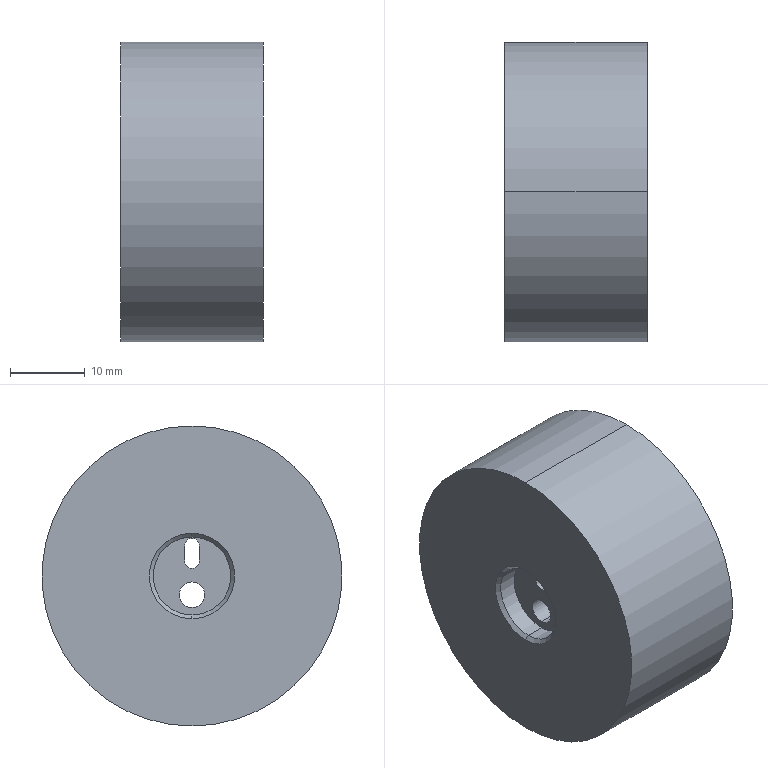Part | SolidWorks | features ICE 3, Chamfer 2, HoleWzd 1, Revolution 1 | 1 solid | 28 faces | box 19 x 40 x 40 mm | volume 21751 mm3 | plane 15 | cylinder 11 | cone 2 | commonest cylinder face diameters 2 x3 3.4 x2 6.5 x2 10.4 x2 40 x2
STEP:
#1=CARTESIAN_POINT('',(0.5,0.,-5.2));
#2=VERTEX_POINT('',#1);
#3=CARTESIAN_POINT('',(0.5,0.,5.2));
#4=VERTEX_POINT('',#3);
#5=CARTESIAN_POINT('',(0.5,0.,0.));
#6=DIRECTION('',(-1.,0.,0.));
#7=DIRECTION('',(0.,0.,1.));
#8=AXIS2_PLACEMENT_3D('',#5,#6,#7);
#9=CIRCLE('',#8,5.2);
#10=EDGE_CURVE('',#2,#4,#9,.T.);
#11=ORIENTED_EDGE('',*,*,#10,.F.);
#12=CARTESIAN_POINT('',(0.,0.,-5.7));
#13=VERTEX_POINT('',#12);
#14=CARTESIAN_POINT('',(0.5,0.,-5.2));
#15=DIRECTION('',(-0.7071,0.,-0.7071));
#16=VECTOR('',#15,1000.);
#17=LINE('',#14,#16);
#18=EDGE_CURVE('',#2,#13,#17,.T.);
#19=ORIENTED_EDGE('',*,*,#18,.T.);
#20=CARTESIAN_POINT('',(0.,0.,5.7));
#21=VERTEX_POINT('',#20);
#22=CARTESIAN_POINT('',(0.,0.,0.));
#23=DIRECTION('',(1.,0.,0.));
#24=DIRECTION('',(0.,0.,1.));
#25=AXIS2_PLACEMENT_3D('',#22,#23,#24);
#26=CIRCLE('',#25,5.7);
#27=EDGE_CURVE('',#21,#13,#26,.T.);
#28=ORIENTED_EDGE('',*,*,#27,.F.);
#29=CARTESIAN_POINT('',(0.5,0.,5.2));
#30=DIRECTION('',(-0.7071,0.,0.7071));
#31=VECTOR('',#30,1000.);
#32=LINE('',#29,#31);
#33=EDGE_CURVE('',#4,#21,#32,.T.);
#34=ORIENTED_EDGE('',*,*,#33,.F.);
#35=EDGE_LOOP('',(#11,#19,#28,#34));
#36=FACE_OUTER_BOUND('',#35,.T.);
#37=CARTESIAN_POINT('',(0.5,0.,0.));
#38=DIRECTION('',(-1.,0.,0.));
#39=DIRECTION('',(0.,0.,1.));
#40=AXIS2_PLACEMENT_3D('',#37,#38,#39);
#41=CONICAL_SURFACE('',#40,5.2,0.7854);
#42=ADVANCED_FACE('',(#36),#41,.F.);
#43=CARTESIAN_POINT('',(3.,0.,-5.2));
#44=VERTEX_POINT('',#43);
#45=CARTESIAN_POINT('',(3.,0.,5.2));
#46=VERTEX_POINT('',#45);
#47=CARTESIAN_POINT('',(3.,0.,0.));
#48=DIRECTION('',(-1.,0.,0.));
#49=DIRECTION('',(0.,0.,1.));
#50=AXIS2_PLACEMENT_3D('',#47,#48,#49);
#51=CIRCLE('',#50,5.2);
#52=EDGE_CURVE('',#44,#46,#51,.T.);
#53=ORIENTED_EDGE('',*,*,#52,.F.);
#54=CARTESIAN_POINT('',(3.,0.,-5.2));
#55=DIRECTION('',(-1.,0.,0.));
#56=VECTOR('',#55,1000.);
#57=LINE('',#54,#56);
#58=EDGE_CURVE('',#44,#2,#57,.T.);
#59=ORIENTED_EDGE('',*,*,#58,.T.);
#60=ORIENTED_EDGE('',*,*,#10,.T.);
#61=CARTESIAN_POINT('',(3.,0.,5.2));
#62=DIRECTION('',(-1.,0.,0.));
#63=VECTOR('',#62,1000.);
#64=LINE('',#61,#63);
#65=EDGE_CURVE('',#46,#4,#64,.T.);
#66=ORIENTED_EDGE('',*,*,#65,.F.);
#67=EDGE_LOOP('',(#53,#59,#60,#66));
#68=FACE_OUTER_BOUND('',#67,.T.);
#69=CARTESIAN_POINT('',(3.,0.,0.));
#70=DIRECTION('',(-1.,0.,0.));
#71=DIRECTION('',(0.,0.,1.));
#72=AXIS2_PLACEMENT_3D('',#69,#70,#71);
#73=CYLINDRICAL_SURFACE('',#72,5.2);
#74=ADVANCED_FACE('',(#68),#73,.F.);
#75=CARTESIAN_POINT('',(6.5,0.,0.75));
#76=VERTEX_POINT('',#75);
#77=CARTESIAN_POINT('',(6.5,0.,-5.75));
#78=VERTEX_POINT('',#77);
#79=CARTESIAN_POINT('',(6.5,0.,-2.5));
#80=DIRECTION('',(1.,0.,0.));
#81=DIRECTION('',(0.,0.,-1.));
#82=AXIS2_PLACEMENT_3D('',#79,#80,#81);
#83=CIRCLE('',#82,3.25);
#84=EDGE_CURVE('',#76,#78,#83,.T.);
#85=ORIENTED_EDGE('',*,*,#84,.F.);
#86=CARTESIAN_POINT('',(10.,0.,0.75));
#87=VERTEX_POINT('',#86);
#88=CARTESIAN_POINT('',(10.,0.,0.75));
#89=DIRECTION('',(1.,0.,0.));
#90=VECTOR('',#89,1000.);
#91=LINE('',#88,#90);
#92=EDGE_CURVE('',#76,#87,#91,.T.);
#93=ORIENTED_EDGE('',*,*,#92,.T.);
#94=CARTESIAN_POINT('',(10.,0.,-5.75));
#95=VERTEX_POINT('',#94);
#96=CARTESIAN_POINT('',(10.,0.,-2.5));
#97=DIRECTION('',(1.,0.,0.));
#98=DIRECTION('',(0.,0.,-1.));
#99=AXIS2_PLACEMENT_3D('',#96,#97,#98);
#100=CIRCLE('',#99,3.25);
#101=EDGE_CURVE('',#87,#95,#100,.T.);
#102=ORIENTED_EDGE('',*,*,#101,.T.);
#103=CARTESIAN_POINT('',(10.,0.,-5.75));
#104=DIRECTION('',(1.,0.,0.));
#105=VECTOR('',#104,1000.);
#106=LINE('',#103,#105);
#107=EDGE_CURVE('',#78,#95,#106,.T.);
#108=ORIENTED_EDGE('',*,*,#107,.F.);
#109=EDGE_LOOP('',(#85,#93,#102,#108));
#110=FACE_OUTER_BOUND('',#109,.T.);
#111=CARTESIAN_POINT('',(10.,0.,-2.5));
#112=DIRECTION('',(1.,0.,0.));
#113=DIRECTION('',(0.,0.,-1.));
#114=AXIS2_PLACEMENT_3D('',#111,#112,#113);
#115=CYLINDRICAL_SURFACE('',#114,3.25);
#116=ADVANCED_FACE('',(#110),#115,.F.);
#117=CARTESIAN_POINT('',(19.,0.,20.));
#118=VERTEX_POINT('',#117);
#119=CARTESIAN_POINT('',(19.,0.,-20.));
#120=VERTEX_POINT('',#119);
#121=CARTESIAN_POINT('',(19.,0.,0.));
#122=DIRECTION('',(-1.,0.,0.));
#123=DIRECTION('',(0.,0.,1.));
#124=AXIS2_PLACEMENT_3D('',#121,#122,#123);
#125=CIRCLE('',#124,20.);
#126=EDGE_CURVE('',#118,#120,#125,.T.);
#127=ORIENTED_EDGE('',*,*,#126,.T.);
#128=CARTESIAN_POINT('',(0.,0.,-20.));
#129=VERTEX_POINT('',#128);
#130=CARTESIAN_POINT('',(0.,0.,-20.));
#131=DIRECTION('',(-1.,0.,0.));
#132=VECTOR('',#131,1000.);
#133=LINE('',#130,#132);
#134=EDGE_CURVE('',#120,#129,#133,.T.);
#135=ORIENTED_EDGE('',*,*,#134,.T.);
#136=CARTESIAN_POINT('',(0.,0.,20.));
#137=VERTEX_POINT('',#136);
#138=CARTESIAN_POINT('',(0.,0.,0.));
#139=DIRECTION('',(-1.,0.,0.));
#140=DIRECTION('',(0.,0.,1.));
#141=AXIS2_PLACEMENT_3D('',#138,#139,#140);
#142=CIRCLE('',#141,20.);
#143=EDGE_CURVE('',#137,#129,#142,.T.);
#144=ORIENTED_EDGE('',*,*,#143,.F.);
#145=CARTESIAN_POINT('',(0.,0.,20.));
#146=DIRECTION('',(-1.,0.,0.));
#147=VECTOR('',#146,1000.);
#148=LINE('',#145,#147);
#149=EDGE_CURVE('',#118,#137,#148,.T.);
#150=ORIENTED_EDGE('',*,*,#149,.F.);
#151=EDGE_LOOP('',(#127,#135,#144,#150));
#152=FACE_OUTER_BOUND('',#151,.T.);
#153=CARTESIAN_POINT('',(0.,0.,0.));
#154=DIRECTION('',(-1.,0.,0.));
#155=DIRECTION('',(0.,0.,1.));
#156=AXIS2_PLACEMENT_3D('',#153,#154,#155);
#157=CYLINDRICAL_SURFACE('',#156,20.);
#158=ADVANCED_FACE('',(#152),#157,.T.);
#159=CARTESIAN_POINT('',(3.,0.,1.));
#160=VERTEX_POINT('',#159);
#161=CARTESIAN_POINT('',(3.,1.,2.));
#162=VERTEX_POINT('',#161);
#163=CARTESIAN_POINT('',(3.,0.,2.));
#164=DIRECTION('',(1.,0.,0.));
#165=DIRECTION('',(0.,0.,1.));
#166=AXIS2_PLACEMENT_3D('',#163,#164,#165);
#167=CIRCLE('',#166,1.);
#168=EDGE_CURVE('',#160,#162,#167,.T.);
#169=ORIENTED_EDGE('',*,*,#168,.F.);
#170=CARTESIAN_POINT('',(10.,0.,1.));
#171=VERTEX_POINT('',#170);
#172=CARTESIAN_POINT('',(0.,0.,1.));
#173=DIRECTION('',(1.,0.,0.));
#174=VECTOR('',#173,1000.);
#175=LINE('',#172,#174);
#176=EDGE_CURVE('',#160,#171,#175,.T.);
#177=ORIENTED_EDGE('',*,*,#176,.T.);
#178=CARTESIAN_POINT('',(10.,1.,2.));
#179=VERTEX_POINT('',#178);
#180=CARTESIAN_POINT('',(10.,0.,2.));
#181=DIRECTION('',(1.,0.,0.));
#182=DIRECTION('',(0.,0.,-1.));
#183=AXIS2_PLACEMENT_3D('',#180,#181,#182);
#184=CIRCLE('',#183,1.);
#185=EDGE_CURVE('',#171,#179,#184,.T.);
#186=ORIENTED_EDGE('',*,*,#185,.T.);
#187=CARTESIAN_POINT('',(0.,1.,2.));
#188=DIRECTION('',(1.,0.,0.));
#189=VECTOR('',#188,1000.);
#190=LINE('',#187,#189);
#191=EDGE_CURVE('',#162,#179,#190,.T.);
#192=ORIENTED_EDGE('',*,*,#191,.F.);
#193=EDGE_LOOP('',(#169,#177,#186,#192));
#194=FACE_OUTER_BOUND('',#193,.T.);
#195=CARTESIAN_POINT('',(0.,0.,2.));
#196=DIRECTION('',(1.,0.,0.));
#197=DIRECTION('',(0.,0.,-1.));
#198=AXIS2_PLACEMENT_3D('',#195,#196,#197);
#199=CYLINDRICAL_SURFACE('',#198,1.);
#200=ADVANCED_FACE('',(#194),#199,.F.);
#201=CARTESIAN_POINT('',(3.,0.,-0.8));
#202=VERTEX_POINT('',#201);
#203=CARTESIAN_POINT('',(3.,0.,-4.2));
#204=VERTEX_POINT('',#203);
#205=CARTESIAN_POINT('',(3.,0.,-2.5));
#206=DIRECTION('',(1.,0.,0.));
#207=DIRECTION('',(0.,0.,1.));
#208=AXIS2_PLACEMENT_3D('',#205,#206,#207);
#209=CIRCLE('',#208,1.7);
#210=EDGE_CURVE('',#202,#204,#209,.T.);
#211=ORIENTED_EDGE('',*,*,#210,.F.);
#212=CARTESIAN_POINT('',(6.5,0.,-0.8));
#213=VERTEX_POINT('',#212);
#214=CARTESIAN_POINT('',(10.,0.,-0.8));
#215=DIRECTION('',(1.,0.,0.));
#216=VECTOR('',#215,1000.);
#217=LINE('',#214,#216);
#218=EDGE_CURVE('',#202,#213,#217,.T.);
#219=ORIENTED_EDGE('',*,*,#218,.T.);
#220=CARTESIAN_POINT('',(6.5,0.,-4.2));
#221=VERTEX_POINT('',#220);
#222=CARTESIAN_POINT('',(6.5,0.,-2.5));
#223=DIRECTION('',(1.,0.,0.));
#224=DIRECTION('',(0.,0.,-1.));
#225=AXIS2_PLACEMENT_3D('',#222,#223,#224);
#226=CIRCLE('',#225,1.7);
#227=EDGE_CURVE('',#213,#221,#226,.T.);
#228=ORIENTED_EDGE('',*,*,#227,.T.);
#229=CARTESIAN_POINT('',(10.,0.,-4.2));
#230=DIRECTION('',(1.,0.,0.));
#231=VECTOR('',#230,1000.);
#232=LINE('',#229,#231);
#233=EDGE_CURVE('',#204,#221,#232,.T.);
#234=ORIENTED_EDGE('',*,*,#233,.F.);
#235=EDGE_LOOP('',(#211,#219,#228,#234));
#236=FACE_OUTER_BOUND('',#235,.T.);
#237=CARTESIAN_POINT('',(10.,0.,-2.5));
#238=DIRECTION('',(1.,0.,0.));
#239=DIRECTION('',(0.,0.,-1.));
#240=AXIS2_PLACEMENT_3D('',#237,#238,#239);
#241=CYLINDRICAL_SURFACE('',#240,1.7);
#242=ADVANCED_FACE('',(#236),#241,.F.);
#243=ORIENTED_EDGE('',*,*,#218,.F.);
#244=CARTESIAN_POINT('',(3.,0.,-2.5));
#245=DIRECTION('',(1.,0.,0.));
#246=DIRECTION('',(0.,0.,1.));
#247=AXIS2_PLACEMENT_3D('',#244,#245,#246);
#248=CIRCLE('',#247,1.7);
#249=EDGE_CURVE('',#204,#202,#248,.T.);
#250=ORIENTED_EDGE('',*,*,#249,.F.);
#251=ORIENTED_EDGE('',*,*,#233,.T.);
#252=CARTESIAN_POINT('',(6.5,0.,-2.5));
#253=DIRECTION('',(1.,0.,0.));
#254=DIRECTION('',(0.,0.,-1.));
#255=AXIS2_PLACEMENT_3D('',#252,#253,#254);
#256=CIRCLE('',#255,1.7);
#257=EDGE_CURVE('',#221,#213,#256,.T.);
#258=ORIENTED_EDGE('',*,*,#257,.T.);
#259=EDGE_LOOP('',(#243,#250,#251,#258));
#260=FACE_OUTER_BOUND('',#259,.T.);
#261=CARTESIAN_POINT('',(10.,0.,-2.5));
#262=DIRECTION('',(1.,0.,0.));
#263=DIRECTION('',(0.,0.,-1.));
#264=AXIS2_PLACEMENT_3D('',#261,#262,#263);
#265=CYLINDRICAL_SURFACE('',#264,1.7);
#266=ADVANCED_FACE('',(#260),#265,.F.);
#267=ORIENTED_EDGE('',*,*,#176,.F.);
#268=CARTESIAN_POINT('',(3.,-1.,2.));
#269=VERTEX_POINT('',#268);
#270=CARTESIAN_POINT('',(3.,0.,2.));
#271=DIRECTION('',(1.,0.,0.));
#272=DIRECTION('',(0.,0.,1.));
#273=AXIS2_PLACEMENT_3D('',#270,#271,#272);
#274=CIRCLE('',#273,1.);
#275=EDGE_CURVE('',#269,#160,#274,.T.);
#276=ORIENTED_EDGE('',*,*,#275,.F.);
#277=CARTESIAN_POINT('',(10.,-1.,2.));
#278=VERTEX_POINT('',#277);
#279=CARTESIAN_POINT('',(0.,-1.,2.));
#280=DIRECTION('',(1.,0.,0.));
#281=VECTOR('',#280,1000.);
#282=LINE('',#279,#281);
#283=EDGE_CURVE('',#269,#278,#282,.T.);
#284=ORIENTED_EDGE('',*,*,#283,.T.);
#285=CARTESIAN_POINT('',(10.,0.,2.));
#286=DIRECTION('',(1.,0.,0.));
#287=DIRECTION('',(0.,0.,-1.));
#288=AXIS2_PLACEMENT_3D('',#285,#286,#287);
#289=CIRCLE('',#288,1.);
#290=EDGE_CURVE('',#278,#171,#289,.T.);
#291=ORIENTED_EDGE('',*,*,#290,.T.);
#292=EDGE_LOOP('',(#267,#276,#284,#291));
#293=FACE_OUTER_BOUND('',#292,.T.);
#294=CARTESIAN_POINT('',(0.,0.,2.));
#295=DIRECTION('',(1.,0.,0.));
#296=DIRECTION('',(0.,0.,-1.));
#297=AXIS2_PLACEMENT_3D('',#294,#295,#296);
#298=CYLINDRICAL_SURFACE('',#297,1.);
#299=ADVANCED_FACE('',(#293),#298,.F.);
#300=CARTESIAN_POINT('',(3.,-1.,4.));
#301=VERTEX_POINT('',#300);
#302=CARTESIAN_POINT('',(3.,-1.,2.));
#303=DIRECTION('',(0.,0.,-1.));
#304=VECTOR('',#303,1000.);
#305=LINE('',#302,#304);
#306=EDGE_CURVE('',#301,#269,#305,.T.);
#307=ORIENTED_EDGE('',*,*,#306,.F.);
#308=CARTESIAN_POINT('',(10.,-1.,4.));
#309=VERTEX_POINT('',#308);
#310=CARTESIAN_POINT('',(0.,-1.,4.));
#311=DIRECTION('',(1.,0.,0.));
#312=VECTOR('',#311,1000.);
#313=LINE('',#310,#312);
#314=EDGE_CURVE('',#301,#309,#313,.T.);
#315=ORIENTED_EDGE('',*,*,#314,.T.);
#316=CARTESIAN_POINT('',(10.,-1.,2.));
#317=DIRECTION('',(0.,0.,-1.));
#318=VECTOR('',#317,1000.);
#319=LINE('',#316,#318);
#320=EDGE_CURVE('',#309,#278,#319,.T.);
#321=ORIENTED_EDGE('',*,*,#320,.T.);
#322=ORIENTED_EDGE('',*,*,#283,.F.);
#323=EDGE_LOOP('',(#307,#315,#321,#322));
#324=FACE_OUTER_BOUND('',#323,.T.);
#325=CARTESIAN_POINT('',(0.,-1.,2.));
#326=DIRECTION('',(0.,-1.,0.));
#327=DIRECTION('',(0.,0.,-1.));
#328=AXIS2_PLACEMENT_3D('',#325,#326,#327);
#329=PLANE('',#328);
#330=ADVANCED_FACE('',(#324),#329,.F.);
#331=CARTESIAN_POINT('',(3.,1.,4.));
#332=VERTEX_POINT('',#331);
#333=CARTESIAN_POINT('',(3.,0.,4.));
#334=DIRECTION('',(1.,0.,0.));
#335=DIRECTION('',(0.,0.,1.));
#336=AXIS2_PLACEMENT_3D('',#333,#334,#335);
#337=CIRCLE('',#336,1.);
#338=EDGE_CURVE('',#332,#301,#337,.T.);
#339=ORIENTED_EDGE('',*,*,#338,.F.);
#340=CARTESIAN_POINT('',(10.,1.,4.));
#341=VERTEX_POINT('',#340);
#342=CARTESIAN_POINT('',(0.,1.,4.));
#343=DIRECTION('',(1.,0.,0.));
#344=VECTOR('',#343,1000.);
#345=LINE('',#342,#344);
#346=EDGE_CURVE('',#332,#341,#345,.T.);
#347=ORIENTED_EDGE('',*,*,#346,.T.);
#348=CARTESIAN_POINT('',(10.,0.,4.));
#349=DIRECTION('',(1.,0.,0.));
#350=DIRECTION('',(0.,0.,-1.));
#351=AXIS2_PLACEMENT_3D('',#348,#349,#350);
#352=CIRCLE('',#351,1.);
#353=EDGE_CURVE('',#341,#309,#352,.T.);
#354=ORIENTED_EDGE('',*,*,#353,.T.);
#355=ORIENTED_EDGE('',*,*,#314,.F.);
#356=EDGE_LOOP('',(#339,#347,#354,#355));
#357=FACE_OUTER_BOUND('',#356,.T.);
#358=CARTESIAN_POINT('',(0.,0.,4.));
#359=DIRECTION('',(1.,0.,0.));
#360=DIRECTION('',(0.,0.,-1.));
#361=AXIS2_PLACEMENT_3D('',#358,#359,#360);
#362=CYLINDRICAL_SURFACE('',#361,1.);
#363=ADVANCED_FACE('',(#357),#362,.F.);
#364=CARTESIAN_POINT('',(3.,1.,2.));
#365=DIRECTION('',(0.,0.,1.));
#366=VECTOR('',#365,1000.);
#367=LINE('',#364,#366);
#368=EDGE_CURVE('',#162,#332,#367,.T.);
#369=ORIENTED_EDGE('',*,*,#368,.F.);
#370=ORIENTED_EDGE('',*,*,#191,.T.);
#371=CARTESIAN_POINT('',(10.,1.,2.));
#372=DIRECTION('',(0.,0.,1.));
#373=VECTOR('',#372,1000.);
#374=LINE('',#371,#373);
#375=EDGE_CURVE('',#179,#341,#374,.T.);
#376=ORIENTED_EDGE('',*,*,#375,.T.);
#377=ORIENTED_EDGE('',*,*,#346,.F.);
#378=EDGE_LOOP('',(#369,#370,#376,#377));
#379=FACE_OUTER_BOUND('',#378,.T.);
#380=CARTESIAN_POINT('',(0.,1.,2.));
#381=DIRECTION('',(0.,1.,0.));
#382=DIRECTION('',(0.,0.,1.));
#383=AXIS2_PLACEMENT_3D('',#380,#381,#382);
#384=PLANE('',#383);
#385=ADVANCED_FACE('',(#379),#384,.F.);
#386=ORIENTED_EDGE('',*,*,#27,.T.);
#387=CARTESIAN_POINT('',(0.,0.,0.));
#388=DIRECTION('',(1.,0.,0.));
#389=DIRECTION('',(0.,0.,1.));
#390=AXIS2_PLACEMENT_3D('',#387,#388,#389);
#391=CIRCLE('',#390,5.7);
#392=EDGE_CURVE('',#13,#21,#391,.T.);
#393=ORIENTED_EDGE('',*,*,#392,.T.);
#394=EDGE_LOOP('',(#386,#393));
#395=FACE_BOUND('',#394,.T.);
#396=ORIENTED_EDGE('',*,*,#143,.T.);
#397=CARTESIAN_POINT('',(0.,0.,0.));
#398=DIRECTION('',(-1.,0.,0.));
#399=DIRECTION('',(0.,0.,1.));
#400=AXIS2_PLACEMENT_3D('',#397,#398,#399);
#401=CIRCLE('',#400,20.);
#402=EDGE_CURVE('',#129,#137,#401,.T.);
#403=ORIENTED_EDGE('',*,*,#402,.T.);
#404=EDGE_LOOP('',(#396,#403));
#405=FACE_OUTER_BOUND('',#404,.T.);
#406=CARTESIAN_POINT('',(0.,0.,0.));
#407=DIRECTION('',(-1.,0.,0.));
#408=DIRECTION('',(0.,0.,1.));
#409=AXIS2_PLACEMENT_3D('',#406,#407,#408);
#410=PLANE('',#409);
#411=ADVANCED_FACE('',(#395,#405),#410,.T.);
#412=ORIENTED_EDGE('',*,*,#134,.F.);
#413=CARTESIAN_POINT('',(19.,0.,0.));
#414=DIRECTION('',(-1.,0.,0.));
#415=DIRECTION('',(0.,0.,1.));
#416=AXIS2_PLACEMENT_3D('',#413,#414,#415);
#417=CIRCLE('',#416,20.);
#418=EDGE_CURVE('',#120,#118,#417,.T.);
#419=ORIENTED_EDGE('',*,*,#418,.T.);
#420=ORIENTED_EDGE('',*,*,#149,.T.);
#421=ORIENTED_EDGE('',*,*,#402,.F.);
#422=EDGE_LOOP('',(#412,#419,#420,#421));
#423=FACE_OUTER_BOUND('',#422,.T.);
#424=CARTESIAN_POINT('',(0.,0.,0.));
#425=DIRECTION('',(-1.,0.,0.));
#426=DIRECTION('',(0.,0.,1.));
#427=AXIS2_PLACEMENT_3D('',#424,#425,#426);
#428=CYLINDRICAL_SURFACE('',#427,20.);
#429=ADVANCED_FACE('',(#423),#428,.T.);
#430=CARTESIAN_POINT('',(19.,7.75,7.75));
#431=VERTEX_POINT('',#430);
#432=CARTESIAN_POINT('',(19.,7.75,-7.75));
#433=VERTEX_POINT('',#432);
#434=CARTESIAN_POINT('',(19.,7.75,-6.75));
#435=DIRECTION('',(0.,0.,-1.));
#436=VECTOR('',#435,1000.);
#437=LINE('',#434,#436);
#438=EDGE_CURVE('',#431,#433,#437,.T.);
#439=ORIENTED_EDGE('',*,*,#438,.T.);
#440=CARTESIAN_POINT('',(19.,-7.75,-7.75));
#441=VERTEX_POINT('',#440);
#442=CARTESIAN_POINT('',(19.,-6.75,-7.75));
#443=DIRECTION('',(0.,-1.,0.));
#444=VECTOR('',#443,1000.);
#445=LINE('',#442,#444);
#446=EDGE_CURVE('',#433,#441,#445,.T.);
#447=ORIENTED_EDGE('',*,*,#446,.T.);
#448=CARTESIAN_POINT('',(19.,-7.75,7.75));
#449=VERTEX_POINT('',#448);
#450=CARTESIAN_POINT('',(19.,-7.75,6.75));
#451=DIRECTION('',(0.,0.,1.));
#452=VECTOR('',#451,1000.);
#453=LINE('',#450,#452);
#454=EDGE_CURVE('',#441,#449,#453,.T.);
#455=ORIENTED_EDGE('',*,*,#454,.T.);
#456=CARTESIAN_POINT('',(19.,6.75,7.75));
#457=DIRECTION('',(0.,1.,0.));
#458=VECTOR('',#457,1000.);
#459=LINE('',#456,#458);
#460=EDGE_CURVE('',#449,#431,#459,.T.);
#461=ORIENTED_EDGE('',*,*,#460,.T.);
#462=EDGE_LOOP('',(#439,#447,#455,#461));
#463=FACE_BOUND('',#462,.T.);
#464=ORIENTED_EDGE('',*,*,#126,.F.);
#465=ORIENTED_EDGE('',*,*,#418,.F.);
#466=EDGE_LOOP('',(#464,#465));
#467=FACE_OUTER_BOUND('',#466,.T.);
#468=CARTESIAN_POINT('',(19.,0.,0.));
#469=DIRECTION('',(1.,0.,0.));
#470=DIRECTION('',(0.,0.,-1.));
#471=AXIS2_PLACEMENT_3D('',#468,#469,#470);
#472=PLANE('',#471);
#473=ADVANCED_FACE('',(#463,#467),#472,.T.);
#474=CARTESIAN_POINT('',(10.,6.75,6.75));
#475=VERTEX_POINT('',#474);
#476=CARTESIAN_POINT('',(18.,6.75,6.75));
#477=VERTEX_POINT('',#476);
#478=CARTESIAN_POINT('',(10.,6.75,6.75));
#479=DIRECTION('',(1.,0.,0.));
#480=VECTOR('',#479,1000.);
#481=LINE('',#478,#480);
#482=EDGE_CURVE('',#475,#477,#481,.T.);
#483=ORIENTED_EDGE('',*,*,#482,.T.);
#484=CARTESIAN_POINT('',(18.,-6.75,6.75));
#485=VERTEX_POINT('',#484);
#486=CARTESIAN_POINT('',(18.,-6.75,6.75));
#487=DIRECTION('',(0.,-1.,0.));
#488=VECTOR('',#487,1000.);
#489=LINE('',#486,#488);
#490=EDGE_CURVE('',#477,#485,#489,.T.);
#491=ORIENTED_EDGE('',*,*,#490,.T.);
#492=CARTESIAN_POINT('',(10.,-6.75,6.75));
#493=VERTEX_POINT('',#492);
#494=CARTESIAN_POINT('',(10.,-6.75,6.75));
#495=DIRECTION('',(1.,0.,0.));
#496=VECTOR('',#495,1000.);
#497=LINE('',#494,#496);
#498=EDGE_CURVE('',#493,#485,#497,.T.);
#499=ORIENTED_EDGE('',*,*,#498,.F.);
#500=CARTESIAN_POINT('',(10.,-6.75,6.75));
#501=DIRECTION('',(0.,-1.,0.));
#502=VECTOR('',#501,1000.);
#503=LINE('',#500,#502);
#504=EDGE_CURVE('',#475,#493,#503,.T.);
#505=ORIENTED_EDGE('',*,*,#504,.F.);
#506=EDGE_LOOP('',(#483,#491,#499,#505));
#507=FACE_OUTER_BOUND('',#506,.T.);
#508=CARTESIAN_POINT('',(10.,-6.75,6.75));
#509=DIRECTION('',(0.,0.,1.));
#510=DIRECTION('',(1.,0.,0.));
#511=AXIS2_PLACEMENT_3D('',#508,#509,#510);
#512=PLANE('',#511);
#513=ADVANCED_FACE('',(#507),#512,.F.);
#514=CARTESIAN_POINT('',(10.,6.75,-6.75));
#515=VERTEX_POINT('',#514);
#516=CARTESIAN_POINT('',(18.,6.75,-6.75));
#517=VERTEX_POINT('',#516);
#518=CARTESIAN_POINT('',(10.,6.75,-6.75));
#519=DIRECTION('',(1.,0.,0.));
#520=VECTOR('',#519,1000.);
#521=LINE('',#518,#520);
#522=EDGE_CURVE('',#515,#517,#521,.T.);
#523=ORIENTED_EDGE('',*,*,#522,.T.);
#524=CARTESIAN_POINT('',(18.,6.75,6.75));
#525=DIRECTION('',(0.,0.,1.));
#526=VECTOR('',#525,1000.);
#527=LINE('',#524,#526);
#528=EDGE_CURVE('',#517,#477,#527,.T.);
#529=ORIENTED_EDGE('',*,*,#528,.T.);
#530=ORIENTED_EDGE('',*,*,#482,.F.);
#531=CARTESIAN_POINT('',(10.,6.75,-6.75));
#532=DIRECTION('',(0.,0.,1.));
#533=VECTOR('',#532,1000.);
#534=LINE('',#531,#533);
#535=EDGE_CURVE('',#515,#475,#534,.T.);
#536=ORIENTED_EDGE('',*,*,#535,.F.);
#537=EDGE_LOOP('',(#523,#529,#530,#536));
#538=FACE_OUTER_BOUND('',#537,.T.);
#539=CARTESIAN_POINT('',(10.,6.75,-6.75));
#540=DIRECTION('',(0.,1.,0.));
#541=DIRECTION('',(0.,0.,1.));
#542=AXIS2_PLACEMENT_3D('',#539,#540,#541);
#543=PLANE('',#542);
#544=ADVANCED_FACE('',(#538),#543,.F.);
#545=CARTESIAN_POINT('',(10.,-6.75,-6.75));
#546=VERTEX_POINT('',#545);
#547=CARTESIAN_POINT('',(18.,-6.75,-6.75));
#548=VERTEX_POINT('',#547);
#549=CARTESIAN_POINT('',(10.,-6.75,-6.75));
#550=DIRECTION('',(1.,0.,0.));
#551=VECTOR('',#550,1000.);
#552=LINE('',#549,#551);
#553=EDGE_CURVE('',#546,#548,#552,.T.);
#554=ORIENTED_EDGE('',*,*,#553,.T.);
#555=CARTESIAN_POINT('',(18.,6.75,-6.75));
#556=DIRECTION('',(0.,1.,0.));
#557=VECTOR('',#556,1000.);
#558=LINE('',#555,#557);
#559=EDGE_CURVE('',#548,#517,#558,.T.);
#560=ORIENTED_EDGE('',*,*,#559,.T.);
#561=ORIENTED_EDGE('',*,*,#522,.F.);
#562=CARTESIAN_POINT('',(10.,-6.75,-6.75));
#563=DIRECTION('',(0.,1.,0.));
#564=VECTOR('',#563,1000.);
#565=LINE('',#562,#564);
#566=EDGE_CURVE('',#546,#515,#565,.T.);
#567=ORIENTED_EDGE('',*,*,#566,.F.);
#568=EDGE_LOOP('',(#554,#560,#561,#567));
#569=FACE_OUTER_BOUND('',#568,.T.);
#570=CARTESIAN_POINT('',(10.,-6.75,-6.75));
#571=DIRECTION('',(0.,0.,-1.));
#572=DIRECTION('',(-1.,0.,0.));
#573=AXIS2_PLACEMENT_3D('',#570,#571,#572);
#574=PLANE('',#573);
#575=ADVANCED_FACE('',(#569),#574,.F.);
#576=ORIENTED_EDGE('',*,*,#498,.T.);
#577=CARTESIAN_POINT('',(18.,-6.75,-6.75));
#578=DIRECTION('',(0.,0.,-1.));
#579=VECTOR('',#578,1000.);
#580=LINE('',#577,#579);
#581=EDGE_CURVE('',#485,#548,#580,.T.);
#582=ORIENTED_EDGE('',*,*,#581,.T.);
#583=ORIENTED_EDGE('',*,*,#553,.F.);
#584=CARTESIAN_POINT('',(10.,-6.75,-6.75));
#585=DIRECTION('',(0.,0.,-1.));
#586=VECTOR('',#585,1000.);
#587=LINE('',#584,#586);
#588=EDGE_CURVE('',#493,#546,#587,.T.);
#589=ORIENTED_EDGE('',*,*,#588,.F.);
#590=EDGE_LOOP('',(#576,#582,#583,#589));
#591=FACE_OUTER_BOUND('',#590,.T.);
#592=CARTESIAN_POINT('',(10.,-6.75,-6.75));
#593=DIRECTION('',(0.,-1.,0.));
#594=DIRECTION('',(0.,0.,-1.));
#595=AXIS2_PLACEMENT_3D('',#592,#593,#594);
#596=PLANE('',#595);
#597=ADVANCED_FACE('',(#591),#596,.F.);
#598=ORIENTED_EDGE('',*,*,#290,.F.);
#599=ORIENTED_EDGE('',*,*,#320,.F.);
#600=ORIENTED_EDGE('',*,*,#353,.F.);
#601=ORIENTED_EDGE('',*,*,#375,.F.);
#602=ORIENTED_EDGE('',*,*,#185,.F.);
#603=EDGE_LOOP('',(#598,#599,#600,#601,#602));
#604=FACE_BOUND('',#603,.T.);
#605=CARTESIAN_POINT('',(10.,0.,-2.5));
#606=DIRECTION('',(1.,0.,0.));
#607=DIRECTION('',(0.,0.,-1.));
#608=AXIS2_PLACEMENT_3D('',#605,#606,#607);
#609=CIRCLE('',#608,3.25);
#610=EDGE_CURVE('',#95,#87,#609,.T.);
#611=ORIENTED_EDGE('',*,*,#610,.F.);
#612=ORIENTED_EDGE('',*,*,#101,.F.);
#613=EDGE_LOOP('',(#611,#612));
#614=FACE_BOUND('',#613,.T.);
#615=ORIENTED_EDGE('',*,*,#504,.T.);
#616=ORIENTED_EDGE('',*,*,#588,.T.);
#617=ORIENTED_EDGE('',*,*,#566,.T.);
#618=ORIENTED_EDGE('',*,*,#535,.T.);
#619=EDGE_LOOP('',(#615,#616,#617,#618));
#620=FACE_OUTER_BOUND('',#619,.T.);
#621=CARTESIAN_POINT('',(10.,6.75,6.75));
#622=DIRECTION('',(1.,0.,0.));
#623=DIRECTION('',(0.,0.,-1.));
#624=AXIS2_PLACEMENT_3D('',#621,#622,#623);
#625=PLANE('',#624);
#626=ADVANCED_FACE('',(#604,#614,#620),#625,.T.);
#627=ORIENTED_EDGE('',*,*,#257,.F.);
#628=ORIENTED_EDGE('',*,*,#227,.F.);
#629=EDGE_LOOP('',(#627,#628));
#630=FACE_BOUND('',#629,.T.);
#631=CARTESIAN_POINT('',(6.5,0.,-2.5));
#632=DIRECTION('',(1.,0.,0.));
#633=DIRECTION('',(0.,0.,-1.));
#634=AXIS2_PLACEMENT_3D('',#631,#632,#633);
#635=CIRCLE('',#634,3.25);
#636=EDGE_CURVE('',#78,#76,#635,.T.);
#637=ORIENTED_EDGE('',*,*,#636,.T.);
#638=ORIENTED_EDGE('',*,*,#84,.T.);
#639=EDGE_LOOP('',(#637,#638));
#640=FACE_OUTER_BOUND('',#639,.T.);
#641=CARTESIAN_POINT('',(6.5,1.7,-2.5));
#642=DIRECTION('',(-1.,0.,0.));
#643=DIRECTION('',(0.,0.,1.));
#644=AXIS2_PLACEMENT_3D('',#641,#642,#643);
#645=PLANE('',#644);
#646=ADVANCED_FACE('',(#630,#640),#645,.F.);
#647=ORIENTED_EDGE('',*,*,#92,.F.);
#648=ORIENTED_EDGE('',*,*,#636,.F.);
#649=ORIENTED_EDGE('',*,*,#107,.T.);
#650=ORIENTED_EDGE('',*,*,#610,.T.);
#651=EDGE_LOOP('',(#647,#648,#649,#650));
#652=FACE_OUTER_BOUND('',#651,.T.);
#653=CARTESIAN_POINT('',(10.,0.,-2.5));
#654=DIRECTION('',(1.,0.,0.));
#655=DIRECTION('',(0.,0.,-1.));
#656=AXIS2_PLACEMENT_3D('',#653,#654,#655);
#657=CYLINDRICAL_SURFACE('',#656,3.25);
#658=ADVANCED_FACE('',(#652),#657,.F.);
#659=CARTESIAN_POINT('',(3.,0.,0.));
#660=DIRECTION('',(-1.,0.,0.));
#661=DIRECTION('',(0.,0.,1.));
#662=AXIS2_PLACEMENT_3D('',#659,#660,#661);
#663=CIRCLE('',#662,5.2);
#664=EDGE_CURVE('',#46,#44,#663,.T.);
#665=ORIENTED_EDGE('',*,*,#664,.T.);
#666=ORIENTED_EDGE('',*,*,#52,.T.);
#667=EDGE_LOOP('',(#665,#666));
#668=FACE_OUTER_BOUND('',#667,.T.);
#669=ORIENTED_EDGE('',*,*,#275,.T.);
#670=ORIENTED_EDGE('',*,*,#168,.T.);
#671=ORIENTED_EDGE('',*,*,#368,.T.);
#672=ORIENTED_EDGE('',*,*,#338,.T.);
#673=ORIENTED_EDGE('',*,*,#306,.T.);
#674=EDGE_LOOP('',(#669,#670,#671,#672,#673));
#675=FACE_BOUND('',#674,.T.);
#676=ORIENTED_EDGE('',*,*,#249,.T.);
#677=ORIENTED_EDGE('',*,*,#210,.T.);
#678=EDGE_LOOP('',(#676,#677));
#679=FACE_BOUND('',#678,.T.);
#680=CARTESIAN_POINT('',(3.,0.,0.));
#681=DIRECTION('',(-1.,0.,0.));
#682=DIRECTION('',(0.,0.,1.));
#683=AXIS2_PLACEMENT_3D('',#680,#681,#682);
#684=PLANE('',#683);
#685=ADVANCED_FACE('',(#668,#675,#679),#684,.T.);
#686=ORIENTED_EDGE('',*,*,#58,.F.);
#687=ORIENTED_EDGE('',*,*,#664,.F.);
#688=ORIENTED_EDGE('',*,*,#65,.T.);
#689=CARTESIAN_POINT('',(0.5,0.,0.));
#690=DIRECTION('',(-1.,0.,0.));
#691=DIRECTION('',(0.,0.,1.));
#692=AXIS2_PLACEMENT_3D('',#689,#690,#691);
#693=CIRCLE('',#692,5.2);
#694=EDGE_CURVE('',#4,#2,#693,.T.);
#695=ORIENTED_EDGE('',*,*,#694,.T.);
#696=EDGE_LOOP('',(#686,#687,#688,#695));
#697=FACE_OUTER_BOUND('',#696,.T.);
#698=CARTESIAN_POINT('',(3.,0.,0.));
#699=DIRECTION('',(-1.,0.,0.));
#700=DIRECTION('',(0.,0.,1.));
#701=AXIS2_PLACEMENT_3D('',#698,#699,#700);
#702=CYLINDRICAL_SURFACE('',#701,5.2);
#703=ADVANCED_FACE('',(#697),#702,.F.);
#704=ORIENTED_EDGE('',*,*,#18,.F.);
#705=ORIENTED_EDGE('',*,*,#694,.F.);
#706=ORIENTED_EDGE('',*,*,#33,.T.);
#707=ORIENTED_EDGE('',*,*,#392,.F.);
#708=EDGE_LOOP('',(#704,#705,#706,#707));
#709=FACE_OUTER_BOUND('',#708,.T.);
#710=CARTESIAN_POINT('',(0.5,0.,0.));
#711=DIRECTION('',(-1.,0.,0.));
#712=DIRECTION('',(0.,0.,1.));
#713=AXIS2_PLACEMENT_3D('',#710,#711,#712);
#714=CONICAL_SURFACE('',#713,5.2,0.7854);
#715=ADVANCED_FACE('',(#709),#714,.F.);
#716=CARTESIAN_POINT('',(13.5,2.25,2.25));
#717=DIRECTION('',(-0.5774,-0.5774,-0.5774));
#718=VECTOR('',#717,1000.);
#719=LINE('',#716,#718);
#720=EDGE_CURVE('',#431,#477,#719,.T.);
#721=ORIENTED_EDGE('',*,*,#720,.F.);
#722=ORIENTED_EDGE('',*,*,#460,.F.);
#723=CARTESIAN_POINT('',(13.5,-2.25,2.25));
#724=DIRECTION('',(0.5774,-0.5774,0.5774));
#725=VECTOR('',#724,1000.);
#726=LINE('',#723,#725);
#727=EDGE_CURVE('',#485,#449,#726,.T.);
#728=ORIENTED_EDGE('',*,*,#727,.F.);
#729=ORIENTED_EDGE('',*,*,#490,.F.);
#730=EDGE_LOOP('',(#721,#722,#728,#729));
#731=FACE_OUTER_BOUND('',#730,.T.);
#732=CARTESIAN_POINT('',(18.,-6.75,6.75));
#733=DIRECTION('',(0.7071,0.,-0.7071));
#734=DIRECTION('',(-0.7071,0.,-0.7071));
#735=AXIS2_PLACEMENT_3D('',#732,#733,#734);
#736=PLANE('',#735);
#737=ADVANCED_FACE('',(#731),#736,.T.);
#738=ORIENTED_EDGE('',*,*,#727,.T.);
#739=ORIENTED_EDGE('',*,*,#454,.F.);
#740=CARTESIAN_POINT('',(18.,-6.75,-6.75));
#741=DIRECTION('',(0.5774,-0.5774,-0.5774));
#742=VECTOR('',#741,1000.);
#743=LINE('',#740,#742);
#744=EDGE_CURVE('',#548,#441,#743,.T.);
#745=ORIENTED_EDGE('',*,*,#744,.F.);
#746=ORIENTED_EDGE('',*,*,#581,.F.);
#747=EDGE_LOOP('',(#738,#739,#745,#746));
#748=FACE_OUTER_BOUND('',#747,.T.);
#749=CARTESIAN_POINT('',(18.,-6.75,-6.75));
#750=DIRECTION('',(0.7071,0.7071,0.));
#751=DIRECTION('',(-0.7071,0.7071,0.));
#752=AXIS2_PLACEMENT_3D('',#749,#750,#751);
#753=PLANE('',#752);
#754=ADVANCED_FACE('',(#748),#753,.T.);
#755=ORIENTED_EDGE('',*,*,#720,.T.);
#756=ORIENTED_EDGE('',*,*,#528,.F.);
#757=CARTESIAN_POINT('',(13.5,2.25,-2.25));
#758=DIRECTION('',(-0.5774,-0.5774,0.5774));
#759=VECTOR('',#758,1000.);
#760=LINE('',#757,#759);
#761=EDGE_CURVE('',#433,#517,#760,.T.);
#762=ORIENTED_EDGE('',*,*,#761,.F.);
#763=ORIENTED_EDGE('',*,*,#438,.F.);
#764=EDGE_LOOP('',(#755,#756,#762,#763));
#765=FACE_OUTER_BOUND('',#764,.T.);
#766=CARTESIAN_POINT('',(18.,6.75,-6.75));
#767=DIRECTION('',(0.7071,-0.7071,0.));
#768=DIRECTION('',(0.7071,0.7071,0.));
#769=AXIS2_PLACEMENT_3D('',#766,#767,#768);
#770=PLANE('',#769);
#771=ADVANCED_FACE('',(#765),#770,.T.);
#772=ORIENTED_EDGE('',*,*,#744,.T.);
#773=ORIENTED_EDGE('',*,*,#446,.F.);
#774=ORIENTED_EDGE('',*,*,#761,.T.);
#775=ORIENTED_EDGE('',*,*,#559,.F.);
#776=EDGE_LOOP('',(#772,#773,#774,#775));
#777=FACE_OUTER_BOUND('',#776,.T.);
#778=CARTESIAN_POINT('',(18.,-6.75,-6.75));
#779=DIRECTION('',(0.7071,0.,0.7071));
#780=DIRECTION('',(0.7071,0.,-0.7071));
#781=AXIS2_PLACEMENT_3D('',#778,#779,#780);
#782=PLANE('',#781);
#783=ADVANCED_FACE('',(#777),#782,.T.);
#784=CLOSED_SHELL('',(#42,#74,#116,#158,#200,#242,#266,#299,#330,#363,#385,#411,#429,#473,#513,#544,#575,#597,#626,#646,#658,#685,#703,#715,#737,#754,#771,#783));
#785=MANIFOLD_SOLID_BREP('',#784);
#786=CARTESIAN_POINT('',(0.,0.,0.));
#787=DIRECTION('',(0.,0.,1.));
#788=DIRECTION('',(1.,0.,0.));
#789=AXIS2_PLACEMENT_3D('',#786,#787,#788);
#790=(LENGTH_UNIT()NAMED_UNIT(*)SI_UNIT(.MILLI.,.METRE.));
#791=UNCERTAINTY_MEASURE_WITH_UNIT(LENGTH_MEASURE(0.00001),#790,'','');
#792=(NAMED_UNIT(*)PLANE_ANGLE_UNIT()SI_UNIT($,.RADIAN.));
#793=(NAMED_UNIT(*)SI_UNIT($,.STERADIAN.)SOLID_ANGLE_UNIT());
#794=(GEOMETRIC_REPRESENTATION_CONTEXT(3)GLOBAL_UNCERTAINTY_ASSIGNED_CONTEXT((#791))GLOBAL_UNIT_ASSIGNED_CONTEXT((#790,#792,#793))REPRESENTATION_CONTEXT('',''));
#795=ADVANCED_BREP_SHAPE_REPRESENTATION('',(#785,#789),#794);